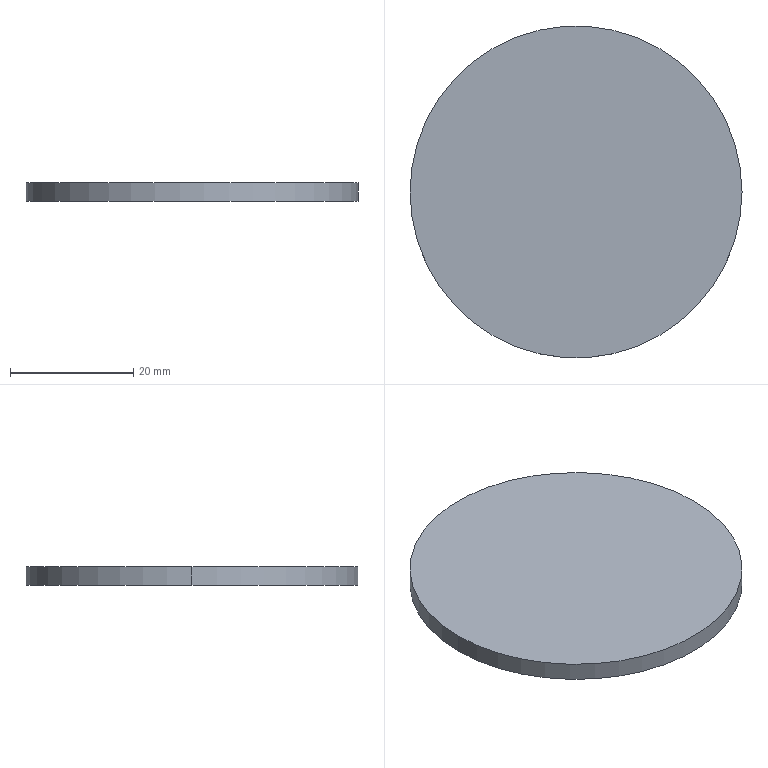Part | SolidWorks | features Extrusion 1 | 1 solid | 4 faces | box 53.9 x 53.9 x 3 mm | volume 6845 mm3 | cylinder 2 | plane 2 | commonest cylinder face diameters 53.9 x2
STEP:
#1=CARTESIAN_POINT('',(26.95,0.,3.));
#2=VERTEX_POINT('',#1);
#3=CARTESIAN_POINT('',(-26.95,0.,3.));
#4=VERTEX_POINT('',#3);
#5=CARTESIAN_POINT('',(0.,0.,3.));
#6=DIRECTION('',(0.,0.,1.));
#7=DIRECTION('',(1.,0.,0.));
#8=AXIS2_PLACEMENT_3D('',#5,#6,#7);
#9=CIRCLE('',#8,26.95);
#10=EDGE_CURVE('',#2,#4,#9,.T.);
#11=ORIENTED_EDGE('',*,*,#10,.F.);
#12=CARTESIAN_POINT('',(26.95,0.,0.));
#13=VERTEX_POINT('',#12);
#14=CARTESIAN_POINT('',(26.95,0.,3.));
#15=DIRECTION('',(0.,0.,-1.));
#16=VECTOR('',#15,1000.);
#17=LINE('',#14,#16);
#18=EDGE_CURVE('',#2,#13,#17,.T.);
#19=ORIENTED_EDGE('',*,*,#18,.T.);
#20=CARTESIAN_POINT('',(-26.95,0.,0.));
#21=VERTEX_POINT('',#20);
#22=CARTESIAN_POINT('',(0.,0.,0.));
#23=DIRECTION('',(0.,0.,1.));
#24=DIRECTION('',(1.,0.,0.));
#25=AXIS2_PLACEMENT_3D('',#22,#23,#24);
#26=CIRCLE('',#25,26.95);
#27=EDGE_CURVE('',#13,#21,#26,.T.);
#28=ORIENTED_EDGE('',*,*,#27,.T.);
#29=CARTESIAN_POINT('',(-26.95,0.,3.));
#30=DIRECTION('',(0.,0.,-1.));
#31=VECTOR('',#30,1000.);
#32=LINE('',#29,#31);
#33=EDGE_CURVE('',#4,#21,#32,.T.);
#34=ORIENTED_EDGE('',*,*,#33,.F.);
#35=EDGE_LOOP('',(#11,#19,#28,#34));
#36=FACE_OUTER_BOUND('',#35,.T.);
#37=CARTESIAN_POINT('',(0.,0.,3.));
#38=DIRECTION('',(0.,0.,-1.));
#39=DIRECTION('',(-1.,0.,0.));
#40=AXIS2_PLACEMENT_3D('',#37,#38,#39);
#41=CYLINDRICAL_SURFACE('',#40,26.95);
#42=ADVANCED_FACE('',(#36),#41,.T.);
#43=ORIENTED_EDGE('',*,*,#18,.F.);
#44=CARTESIAN_POINT('',(0.,0.,3.));
#45=DIRECTION('',(0.,0.,1.));
#46=DIRECTION('',(1.,0.,0.));
#47=AXIS2_PLACEMENT_3D('',#44,#45,#46);
#48=CIRCLE('',#47,26.95);
#49=EDGE_CURVE('',#4,#2,#48,.T.);
#50=ORIENTED_EDGE('',*,*,#49,.F.);
#51=ORIENTED_EDGE('',*,*,#33,.T.);
#52=CARTESIAN_POINT('',(0.,0.,0.));
#53=DIRECTION('',(0.,0.,1.));
#54=DIRECTION('',(1.,0.,0.));
#55=AXIS2_PLACEMENT_3D('',#52,#53,#54);
#56=CIRCLE('',#55,26.95);
#57=EDGE_CURVE('',#21,#13,#56,.T.);
#58=ORIENTED_EDGE('',*,*,#57,.T.);
#59=EDGE_LOOP('',(#43,#50,#51,#58));
#60=FACE_OUTER_BOUND('',#59,.T.);
#61=CARTESIAN_POINT('',(0.,0.,3.));
#62=DIRECTION('',(0.,0.,-1.));
#63=DIRECTION('',(-1.,0.,0.));
#64=AXIS2_PLACEMENT_3D('',#61,#62,#63);
#65=CYLINDRICAL_SURFACE('',#64,26.95);
#66=ADVANCED_FACE('',(#60),#65,.T.);
#67=ORIENTED_EDGE('',*,*,#49,.T.);
#68=ORIENTED_EDGE('',*,*,#10,.T.);
#69=EDGE_LOOP('',(#67,#68));
#70=FACE_OUTER_BOUND('',#69,.T.);
#71=CARTESIAN_POINT('',(0.,0.,3.));
#72=DIRECTION('',(0.,0.,1.));
#73=DIRECTION('',(1.,0.,0.));
#74=AXIS2_PLACEMENT_3D('',#71,#72,#73);
#75=PLANE('',#74);
#76=ADVANCED_FACE('',(#70),#75,.T.);
#77=ORIENTED_EDGE('',*,*,#57,.F.);
#78=ORIENTED_EDGE('',*,*,#27,.F.);
#79=EDGE_LOOP('',(#77,#78));
#80=FACE_OUTER_BOUND('',#79,.T.);
#81=CARTESIAN_POINT('',(0.,0.,0.));
#82=DIRECTION('',(0.,0.,1.));
#83=DIRECTION('',(1.,0.,0.));
#84=AXIS2_PLACEMENT_3D('',#81,#82,#83);
#85=PLANE('',#84);
#86=ADVANCED_FACE('',(#80),#85,.F.);
#87=CLOSED_SHELL('',(#42,#66,#76,#86));
#88=MANIFOLD_SOLID_BREP('',#87);
#89=CARTESIAN_POINT('',(0.,0.,0.));
#90=DIRECTION('',(0.,0.,1.));
#91=DIRECTION('',(1.,0.,0.));
#92=AXIS2_PLACEMENT_3D('',#89,#90,#91);
#93=(LENGTH_UNIT()NAMED_UNIT(*)SI_UNIT(.MILLI.,.METRE.));
#94=UNCERTAINTY_MEASURE_WITH_UNIT(LENGTH_MEASURE(0.00001),#93,'','');
#95=(NAMED_UNIT(*)PLANE_ANGLE_UNIT()SI_UNIT($,.RADIAN.));
#96=(NAMED_UNIT(*)SI_UNIT($,.STERADIAN.)SOLID_ANGLE_UNIT());
#97=(GEOMETRIC_REPRESENTATION_CONTEXT(3)GLOBAL_UNCERTAINTY_ASSIGNED_CONTEXT((#94))GLOBAL_UNIT_ASSIGNED_CONTEXT((#93,#95,#96))REPRESENTATION_CONTEXT('',''));
#98=ADVANCED_BREP_SHAPE_REPRESENTATION('',(#88,#92),#97);